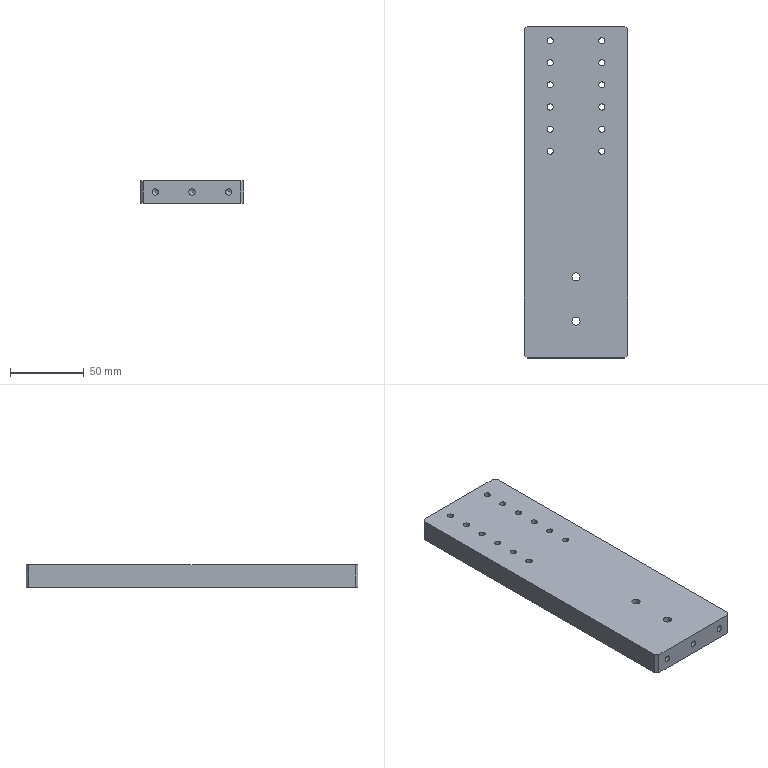Part | NX | 1 solid | 40 faces | box 70 x 225 x 15 mm | volume 210528 mm3 | cylinder 21 | plane 16 | cone 3 | commonest cylinder face diameters 4.2 x15 4 x2 5.5 x2 10 x2
STEP:
#1=CARTESIAN_POINT('',(-33.,112.5,15.));
#2=VERTEX_POINT('',#1);
#3=CARTESIAN_POINT('',(-35.,110.5,15.));
#4=VERTEX_POINT('',#3);
#5=CARTESIAN_POINT('',(-35.,110.5,15.));
#6=DIRECTION('',(-0.7071,-0.7071,0.));
#7=VECTOR('',#6,1000.);
#8=LINE('',#5,#7);
#9=EDGE_CURVE('',#2,#4,#8,.T.);
#10=ORIENTED_EDGE('',*,*,#9,.F.);
#11=CARTESIAN_POINT('',(-33.,112.5,0.));
#12=VERTEX_POINT('',#11);
#13=CARTESIAN_POINT('',(-33.,112.5,15.));
#14=DIRECTION('',(0.,0.,1.));
#15=VECTOR('',#14,1000.);
#16=LINE('',#13,#15);
#17=EDGE_CURVE('',#12,#2,#16,.T.);
#18=ORIENTED_EDGE('',*,*,#17,.F.);
#19=CARTESIAN_POINT('',(-35.,110.5,0.));
#20=VERTEX_POINT('',#19);
#21=CARTESIAN_POINT('',(-72.75,72.75,0.));
#22=DIRECTION('',(0.7071,0.7071,0.));
#23=VECTOR('',#22,1000.);
#24=LINE('',#21,#23);
#25=EDGE_CURVE('',#20,#12,#24,.T.);
#26=ORIENTED_EDGE('',*,*,#25,.F.);
#27=CARTESIAN_POINT('',(-35.,110.5,15.));
#28=DIRECTION('',(0.,0.,-1.));
#29=VECTOR('',#28,1000.);
#30=LINE('',#27,#29);
#31=EDGE_CURVE('',#4,#20,#30,.T.);
#32=ORIENTED_EDGE('',*,*,#31,.F.);
#33=EDGE_LOOP('',(#10,#18,#26,#32));
#34=FACE_BOUND('',#33,.T.);
#35=CARTESIAN_POINT('',(-35.,110.5,15.));
#36=DIRECTION('',(0.7071,-0.7071,0.));
#37=DIRECTION('',(0.,0.,-1.));
#38=AXIS2_PLACEMENT_3D('',#35,#36,#37);
#39=PLANE('',#38);
#40=ADVANCED_FACE('',(#34),#39,.F.);
#41=CARTESIAN_POINT('',(35.,110.5,15.));
#42=VERTEX_POINT('',#41);
#43=CARTESIAN_POINT('',(33.,112.5,15.));
#44=VERTEX_POINT('',#43);
#45=CARTESIAN_POINT('',(33.,112.5,15.));
#46=DIRECTION('',(-0.7071,0.7071,0.));
#47=VECTOR('',#46,1000.);
#48=LINE('',#45,#47);
#49=EDGE_CURVE('',#42,#44,#48,.T.);
#50=ORIENTED_EDGE('',*,*,#49,.F.);
#51=CARTESIAN_POINT('',(35.,110.5,0.));
#52=VERTEX_POINT('',#51);
#53=CARTESIAN_POINT('',(35.,110.5,15.));
#54=DIRECTION('',(0.,0.,1.));
#55=VECTOR('',#54,1000.);
#56=LINE('',#53,#55);
#57=EDGE_CURVE('',#52,#42,#56,.T.);
#58=ORIENTED_EDGE('',*,*,#57,.F.);
#59=CARTESIAN_POINT('',(33.,112.5,0.));
#60=VERTEX_POINT('',#59);
#61=CARTESIAN_POINT('',(72.75,72.75,0.));
#62=DIRECTION('',(0.7071,-0.7071,0.));
#63=VECTOR('',#62,1000.);
#64=LINE('',#61,#63);
#65=EDGE_CURVE('',#60,#52,#64,.T.);
#66=ORIENTED_EDGE('',*,*,#65,.F.);
#67=CARTESIAN_POINT('',(33.,112.5,15.));
#68=DIRECTION('',(0.,0.,-1.));
#69=VECTOR('',#68,1000.);
#70=LINE('',#67,#69);
#71=EDGE_CURVE('',#44,#60,#70,.T.);
#72=ORIENTED_EDGE('',*,*,#71,.F.);
#73=EDGE_LOOP('',(#50,#58,#66,#72));
#74=FACE_BOUND('',#73,.T.);
#75=CARTESIAN_POINT('',(33.,112.5,15.));
#76=DIRECTION('',(-0.7071,-0.7071,0.));
#77=DIRECTION('',(0.,0.,-1.));
#78=AXIS2_PLACEMENT_3D('',#75,#76,#77);
#79=PLANE('',#78);
#80=ADVANCED_FACE('',(#74),#79,.F.);
#81=CARTESIAN_POINT('',(-35.,-110.5,15.));
#82=VERTEX_POINT('',#81);
#83=CARTESIAN_POINT('',(-33.,-112.5,15.));
#84=VERTEX_POINT('',#83);
#85=CARTESIAN_POINT('',(-33.,-112.5,15.));
#86=DIRECTION('',(0.7071,-0.7071,0.));
#87=VECTOR('',#86,1000.);
#88=LINE('',#85,#87);
#89=EDGE_CURVE('',#82,#84,#88,.T.);
#90=ORIENTED_EDGE('',*,*,#89,.F.);
#91=CARTESIAN_POINT('',(-35.,-110.5,0.));
#92=VERTEX_POINT('',#91);
#93=CARTESIAN_POINT('',(-35.,-110.5,15.));
#94=DIRECTION('',(0.,0.,1.));
#95=VECTOR('',#94,1000.);
#96=LINE('',#93,#95);
#97=EDGE_CURVE('',#92,#82,#96,.T.);
#98=ORIENTED_EDGE('',*,*,#97,.F.);
#99=CARTESIAN_POINT('',(-33.,-112.5,0.));
#100=VERTEX_POINT('',#99);
#101=CARTESIAN_POINT('',(-72.75,-72.75,0.));
#102=DIRECTION('',(-0.7071,0.7071,0.));
#103=VECTOR('',#102,1000.);
#104=LINE('',#101,#103);
#105=EDGE_CURVE('',#100,#92,#104,.T.);
#106=ORIENTED_EDGE('',*,*,#105,.F.);
#107=CARTESIAN_POINT('',(-33.,-112.5,15.));
#108=DIRECTION('',(0.,0.,-1.));
#109=VECTOR('',#108,1000.);
#110=LINE('',#107,#109);
#111=EDGE_CURVE('',#84,#100,#110,.T.);
#112=ORIENTED_EDGE('',*,*,#111,.F.);
#113=EDGE_LOOP('',(#90,#98,#106,#112));
#114=FACE_BOUND('',#113,.T.);
#115=CARTESIAN_POINT('',(-33.,-112.5,15.));
#116=DIRECTION('',(0.7071,0.7071,0.));
#117=DIRECTION('',(0.,0.,-1.));
#118=AXIS2_PLACEMENT_3D('',#115,#116,#117);
#119=PLANE('',#118);
#120=ADVANCED_FACE('',(#114),#119,.F.);
#121=CARTESIAN_POINT('',(33.,-112.5,15.));
#122=VERTEX_POINT('',#121);
#123=CARTESIAN_POINT('',(35.,-110.5,15.));
#124=VERTEX_POINT('',#123);
#125=CARTESIAN_POINT('',(35.,-110.5,15.));
#126=DIRECTION('',(0.7071,0.7071,0.));
#127=VECTOR('',#126,1000.);
#128=LINE('',#125,#127);
#129=EDGE_CURVE('',#122,#124,#128,.T.);
#130=ORIENTED_EDGE('',*,*,#129,.F.);
#131=CARTESIAN_POINT('',(33.,-112.5,0.));
#132=VERTEX_POINT('',#131);
#133=CARTESIAN_POINT('',(33.,-112.5,15.));
#134=DIRECTION('',(0.,0.,1.));
#135=VECTOR('',#134,1000.);
#136=LINE('',#133,#135);
#137=EDGE_CURVE('',#132,#122,#136,.T.);
#138=ORIENTED_EDGE('',*,*,#137,.F.);
#139=CARTESIAN_POINT('',(35.,-110.5,0.));
#140=VERTEX_POINT('',#139);
#141=CARTESIAN_POINT('',(72.75,-72.75,0.));
#142=DIRECTION('',(-0.7071,-0.7071,0.));
#143=VECTOR('',#142,1000.);
#144=LINE('',#141,#143);
#145=EDGE_CURVE('',#140,#132,#144,.T.);
#146=ORIENTED_EDGE('',*,*,#145,.F.);
#147=CARTESIAN_POINT('',(35.,-110.5,15.));
#148=DIRECTION('',(0.,0.,-1.));
#149=VECTOR('',#148,1000.);
#150=LINE('',#147,#149);
#151=EDGE_CURVE('',#124,#140,#150,.T.);
#152=ORIENTED_EDGE('',*,*,#151,.F.);
#153=EDGE_LOOP('',(#130,#138,#146,#152));
#154=FACE_BOUND('',#153,.T.);
#155=CARTESIAN_POINT('',(35.,-110.5,15.));
#156=DIRECTION('',(-0.7071,0.7071,0.));
#157=DIRECTION('',(0.,0.,-1.));
#158=AXIS2_PLACEMENT_3D('',#155,#156,#157);
#159=PLANE('',#158);
#160=ADVANCED_FACE('',(#154),#159,.F.);
#161=CARTESIAN_POINT('',(-5.,-57.5,7.));
#162=VERTEX_POINT('',#161);
#163=CARTESIAN_POINT('',(0.,-57.5,7.));
#164=DIRECTION('',(0.,0.,-1.));
#165=DIRECTION('',(-1.,0.,0.));
#166=AXIS2_PLACEMENT_3D('',#163,#164,#165);
#167=CIRCLE('',#166,5.);
#168=EDGE_CURVE('',#162,#162,#167,.T.);
#169=ORIENTED_EDGE('',*,*,#168,.T.);
#170=EDGE_LOOP('',(#169));
#171=FACE_BOUND('',#170,.T.);
#172=CARTESIAN_POINT('',(-2.75,-57.5,7.));
#173=VERTEX_POINT('',#172);
#174=CARTESIAN_POINT('',(0.,-57.5,7.));
#175=DIRECTION('',(0.,0.,-1.));
#176=DIRECTION('',(-1.,0.,0.));
#177=AXIS2_PLACEMENT_3D('',#174,#175,#176);
#178=CIRCLE('',#177,2.75);
#179=EDGE_CURVE('',#173,#173,#178,.T.);
#180=ORIENTED_EDGE('',*,*,#179,.F.);
#181=EDGE_LOOP('',(#180));
#182=FACE_BOUND('',#181,.T.);
#183=CARTESIAN_POINT('',(2.75,-57.5,7.));
#184=DIRECTION('',(0.,0.,1.));
#185=DIRECTION('',(1.,0.,0.));
#186=AXIS2_PLACEMENT_3D('',#183,#184,#185);
#187=PLANE('',#186);
#188=ADVANCED_FACE('',(#171,#182),#187,.F.);
#189=CARTESIAN_POINT('',(5.,-87.5,7.));
#190=VERTEX_POINT('',#189);
#191=CARTESIAN_POINT('',(0.,-87.5,7.));
#192=DIRECTION('',(0.,0.,-1.));
#193=DIRECTION('',(1.,0.,0.));
#194=AXIS2_PLACEMENT_3D('',#191,#192,#193);
#195=CIRCLE('',#194,5.);
#196=EDGE_CURVE('',#190,#190,#195,.T.);
#197=ORIENTED_EDGE('',*,*,#196,.T.);
#198=EDGE_LOOP('',(#197));
#199=FACE_BOUND('',#198,.T.);
#200=CARTESIAN_POINT('',(2.75,-87.5,7.));
#201=VERTEX_POINT('',#200);
#202=CARTESIAN_POINT('',(0.,-87.5,7.));
#203=DIRECTION('',(0.,0.,-1.));
#204=DIRECTION('',(1.,0.,0.));
#205=AXIS2_PLACEMENT_3D('',#202,#203,#204);
#206=CIRCLE('',#205,2.75);
#207=EDGE_CURVE('',#201,#201,#206,.T.);
#208=ORIENTED_EDGE('',*,*,#207,.F.);
#209=EDGE_LOOP('',(#208));
#210=FACE_BOUND('',#209,.T.);
#211=CARTESIAN_POINT('',(2.75,-57.5,7.));
#212=DIRECTION('',(0.,0.,1.));
#213=DIRECTION('',(1.,0.,0.));
#214=AXIS2_PLACEMENT_3D('',#211,#212,#213);
#215=PLANE('',#214);
#216=ADVANCED_FACE('',(#199,#210),#215,.F.);
#217=CARTESIAN_POINT('',(30.,-5.5,3.));
#218=VERTEX_POINT('',#217);
#219=CARTESIAN_POINT('',(28.,-7.5,3.));
#220=VERTEX_POINT('',#219);
#221=CARTESIAN_POINT('',(28.,-5.5,3.));
#222=DIRECTION('',(0.,0.,-1.));
#223=DIRECTION('',(-1.,0.,0.));
#224=AXIS2_PLACEMENT_3D('',#221,#222,#223);
#225=CIRCLE('',#224,2.);
#226=EDGE_CURVE('',#218,#220,#225,.T.);
#227=ORIENTED_EDGE('',*,*,#226,.F.);
#228=CARTESIAN_POINT('',(30.,-5.5,0.));
#229=VERTEX_POINT('',#228);
#230=CARTESIAN_POINT('',(30.,-5.5,3.));
#231=DIRECTION('',(0.,0.,1.));
#232=VECTOR('',#231,1000.);
#233=LINE('',#230,#232);
#234=EDGE_CURVE('',#229,#218,#233,.T.);
#235=ORIENTED_EDGE('',*,*,#234,.F.);
#236=CARTESIAN_POINT('',(28.,-7.5,0.));
#237=VERTEX_POINT('',#236);
#238=CARTESIAN_POINT('',(28.,-5.5,0.));
#239=DIRECTION('',(0.,0.,1.));
#240=DIRECTION('',(-1.,0.,0.));
#241=AXIS2_PLACEMENT_3D('',#238,#239,#240);
#242=CIRCLE('',#241,2.);
#243=EDGE_CURVE('',#237,#229,#242,.T.);
#244=ORIENTED_EDGE('',*,*,#243,.F.);
#245=CARTESIAN_POINT('',(28.,-7.5,0.));
#246=DIRECTION('',(0.,0.,-1.));
#247=VECTOR('',#246,1000.);
#248=LINE('',#245,#247);
#249=EDGE_CURVE('',#220,#237,#248,.T.);
#250=ORIENTED_EDGE('',*,*,#249,.F.);
#251=EDGE_LOOP('',(#227,#235,#244,#250));
#252=FACE_BOUND('',#251,.T.);
#253=CARTESIAN_POINT('',(28.,-5.5,3.));
#254=DIRECTION('',(0.,0.,1.));
#255=DIRECTION('',(1.,0.,0.));
#256=AXIS2_PLACEMENT_3D('',#253,#254,#255);
#257=CYLINDRICAL_SURFACE('',#256,2.);
#258=ADVANCED_FACE('',(#252),#257,.F.);
#259=CARTESIAN_POINT('',(-28.,-7.5,3.));
#260=VERTEX_POINT('',#259);
#261=CARTESIAN_POINT('',(-30.,-5.5,3.));
#262=VERTEX_POINT('',#261);
#263=CARTESIAN_POINT('',(-28.,-5.5,3.));
#264=DIRECTION('',(0.,0.,-1.));
#265=DIRECTION('',(-1.,0.,0.));
#266=AXIS2_PLACEMENT_3D('',#263,#264,#265);
#267=CIRCLE('',#266,2.);
#268=EDGE_CURVE('',#260,#262,#267,.T.);
#269=ORIENTED_EDGE('',*,*,#268,.F.);
#270=CARTESIAN_POINT('',(-28.,-7.5,0.));
#271=VERTEX_POINT('',#270);
#272=CARTESIAN_POINT('',(-28.,-7.5,3.));
#273=DIRECTION('',(0.,0.,1.));
#274=VECTOR('',#273,1000.);
#275=LINE('',#272,#274);
#276=EDGE_CURVE('',#271,#260,#275,.T.);
#277=ORIENTED_EDGE('',*,*,#276,.F.);
#278=CARTESIAN_POINT('',(-30.,-5.5,0.));
#279=VERTEX_POINT('',#278);
#280=CARTESIAN_POINT('',(-28.,-5.5,0.));
#281=DIRECTION('',(0.,0.,1.));
#282=DIRECTION('',(-1.,0.,0.));
#283=AXIS2_PLACEMENT_3D('',#280,#281,#282);
#284=CIRCLE('',#283,2.);
#285=EDGE_CURVE('',#279,#271,#284,.T.);
#286=ORIENTED_EDGE('',*,*,#285,.F.);
#287=CARTESIAN_POINT('',(-30.,-5.5,0.));
#288=DIRECTION('',(0.,0.,-1.));
#289=VECTOR('',#288,1000.);
#290=LINE('',#287,#289);
#291=EDGE_CURVE('',#262,#279,#290,.T.);
#292=ORIENTED_EDGE('',*,*,#291,.F.);
#293=EDGE_LOOP('',(#269,#277,#286,#292));
#294=FACE_BOUND('',#293,.T.);
#295=CARTESIAN_POINT('',(-28.,-5.5,3.));
#296=DIRECTION('',(0.,0.,1.));
#297=DIRECTION('',(1.,0.,0.));
#298=AXIS2_PLACEMENT_3D('',#295,#296,#297);
#299=CYLINDRICAL_SURFACE('',#298,2.);
#300=ADVANCED_FACE('',(#294),#299,.F.);
#301=CARTESIAN_POINT('',(30.,-7.5,0.));
#302=DIRECTION('',(-1.,0.,0.));
#303=VECTOR('',#302,1000.);
#304=LINE('',#301,#303);
#305=EDGE_CURVE('',#237,#271,#304,.T.);
#306=ORIENTED_EDGE('',*,*,#305,.T.);
#307=ORIENTED_EDGE('',*,*,#276,.T.);
#308=CARTESIAN_POINT('',(30.,-7.5,3.));
#309=DIRECTION('',(-1.,0.,0.));
#310=VECTOR('',#309,1000.);
#311=LINE('',#308,#310);
#312=EDGE_CURVE('',#220,#260,#311,.T.);
#313=ORIENTED_EDGE('',*,*,#312,.F.);
#314=ORIENTED_EDGE('',*,*,#249,.T.);
#315=EDGE_LOOP('',(#306,#307,#313,#314));
#316=FACE_BOUND('',#315,.T.);
#317=CARTESIAN_POINT('',(30.,-7.5,3.));
#318=DIRECTION('',(0.,-1.,0.));
#319=DIRECTION('',(1.,0.,0.));
#320=AXIS2_PLACEMENT_3D('',#317,#318,#319);
#321=PLANE('',#320);
#322=ADVANCED_FACE('',(#316),#321,.F.);
#323=CARTESIAN_POINT('',(30.,112.5,0.));
#324=VERTEX_POINT('',#323);
#325=CARTESIAN_POINT('',(30.,0.,0.));
#326=DIRECTION('',(0.,-1.,0.));
#327=VECTOR('',#326,1000.);
#328=LINE('',#325,#327);
#329=EDGE_CURVE('',#324,#229,#328,.T.);
#330=ORIENTED_EDGE('',*,*,#329,.T.);
#331=ORIENTED_EDGE('',*,*,#234,.T.);
#332=CARTESIAN_POINT('',(30.,112.5,3.));
#333=VERTEX_POINT('',#332);
#334=CARTESIAN_POINT('',(30.,232.5,3.));
#335=DIRECTION('',(0.,-1.,0.));
#336=VECTOR('',#335,1000.);
#337=LINE('',#334,#336);
#338=EDGE_CURVE('',#333,#218,#337,.T.);
#339=ORIENTED_EDGE('',*,*,#338,.F.);
#340=CARTESIAN_POINT('',(30.,112.5,15.));
#341=DIRECTION('',(0.,0.,1.));
#342=VECTOR('',#341,1000.);
#343=LINE('',#340,#342);
#344=EDGE_CURVE('',#324,#333,#343,.T.);
#345=ORIENTED_EDGE('',*,*,#344,.F.);
#346=EDGE_LOOP('',(#330,#331,#339,#345));
#347=FACE_BOUND('',#346,.T.);
#348=CARTESIAN_POINT('',(30.,232.5,3.));
#349=DIRECTION('',(1.,0.,0.));
#350=DIRECTION('',(0.,0.,-1.));
#351=AXIS2_PLACEMENT_3D('',#348,#349,#350);
#352=PLANE('',#351);
#353=ADVANCED_FACE('',(#347),#352,.F.);
#354=CARTESIAN_POINT('',(-30.,112.5,3.));
#355=VERTEX_POINT('',#354);
#356=CARTESIAN_POINT('',(-30.,232.5,3.));
#357=DIRECTION('',(0.,1.,0.));
#358=VECTOR('',#357,1000.);
#359=LINE('',#356,#358);
#360=EDGE_CURVE('',#262,#355,#359,.T.);
#361=ORIENTED_EDGE('',*,*,#360,.F.);
#362=ORIENTED_EDGE('',*,*,#291,.T.);
#363=CARTESIAN_POINT('',(-30.,112.5,0.));
#364=VERTEX_POINT('',#363);
#365=CARTESIAN_POINT('',(-30.,232.5,0.));
#366=DIRECTION('',(0.,1.,0.));
#367=VECTOR('',#366,1000.);
#368=LINE('',#365,#367);
#369=EDGE_CURVE('',#279,#364,#368,.T.);
#370=ORIENTED_EDGE('',*,*,#369,.T.);
#371=CARTESIAN_POINT('',(-30.,112.5,15.));
#372=DIRECTION('',(0.,0.,-1.));
#373=VECTOR('',#372,1000.);
#374=LINE('',#371,#373);
#375=EDGE_CURVE('',#355,#364,#374,.T.);
#376=ORIENTED_EDGE('',*,*,#375,.F.);
#377=EDGE_LOOP('',(#361,#362,#370,#376));
#378=FACE_BOUND('',#377,.T.);
#379=CARTESIAN_POINT('',(-30.,232.5,3.));
#380=DIRECTION('',(-1.,0.,0.));
#381=DIRECTION('',(0.,-1.,0.));
#382=AXIS2_PLACEMENT_3D('',#379,#380,#381);
#383=PLANE('',#382);
#384=ADVANCED_FACE('',(#378),#383,.F.);
#385=ORIENTED_EDGE('',*,*,#312,.T.);
#386=ORIENTED_EDGE('',*,*,#268,.T.);
#387=ORIENTED_EDGE('',*,*,#360,.T.);
#388=CARTESIAN_POINT('',(-35.,112.5,3.));
#389=DIRECTION('',(1.,0.,0.));
#390=VECTOR('',#389,1000.);
#391=LINE('',#388,#390);
#392=EDGE_CURVE('',#355,#333,#391,.T.);
#393=ORIENTED_EDGE('',*,*,#392,.T.);
#394=ORIENTED_EDGE('',*,*,#338,.T.);
#395=ORIENTED_EDGE('',*,*,#226,.T.);
#396=EDGE_LOOP('',(#385,#386,#387,#393,#394,#395));
#397=FACE_BOUND('',#396,.T.);
#398=CARTESIAN_POINT('',(-19.6,102.571,3.));
#399=VERTEX_POINT('',#398);
#400=CARTESIAN_POINT('',(-17.5,102.571,3.));
#401=DIRECTION('',(0.,0.,-1.));
#402=DIRECTION('',(-1.,0.,0.));
#403=AXIS2_PLACEMENT_3D('',#400,#401,#402);
#404=CIRCLE('',#403,2.1);
#405=EDGE_CURVE('',#399,#399,#404,.T.);
#406=ORIENTED_EDGE('',*,*,#405,.F.);
#407=EDGE_LOOP('',(#406));
#408=FACE_BOUND('',#407,.T.);
#409=CARTESIAN_POINT('',(15.4,102.571,3.));
#410=VERTEX_POINT('',#409);
#411=CARTESIAN_POINT('',(17.5,102.571,3.));
#412=DIRECTION('',(0.,0.,-1.));
#413=DIRECTION('',(-1.,0.,0.));
#414=AXIS2_PLACEMENT_3D('',#411,#412,#413);
#415=CIRCLE('',#414,2.1);
#416=EDGE_CURVE('',#410,#410,#415,.T.);
#417=ORIENTED_EDGE('',*,*,#416,.F.);
#418=EDGE_LOOP('',(#417));
#419=FACE_BOUND('',#418,.T.);
#420=CARTESIAN_POINT('',(-19.6,87.571,3.));
#421=VERTEX_POINT('',#420);
#422=CARTESIAN_POINT('',(-17.5,87.571,3.));
#423=DIRECTION('',(0.,0.,-1.));
#424=DIRECTION('',(-1.,0.,0.));
#425=AXIS2_PLACEMENT_3D('',#422,#423,#424);
#426=CIRCLE('',#425,2.1);
#427=EDGE_CURVE('',#421,#421,#426,.T.);
#428=ORIENTED_EDGE('',*,*,#427,.F.);
#429=EDGE_LOOP('',(#428));
#430=FACE_BOUND('',#429,.T.);
#431=CARTESIAN_POINT('',(15.4,87.571,3.));
#432=VERTEX_POINT('',#431);
#433=CARTESIAN_POINT('',(17.5,87.571,3.));
#434=DIRECTION('',(0.,0.,-1.));
#435=DIRECTION('',(-1.,0.,0.));
#436=AXIS2_PLACEMENT_3D('',#433,#434,#435);
#437=CIRCLE('',#436,2.1);
#438=EDGE_CURVE('',#432,#432,#437,.T.);
#439=ORIENTED_EDGE('',*,*,#438,.F.);
#440=EDGE_LOOP('',(#439));
#441=FACE_BOUND('',#440,.T.);
#442=CARTESIAN_POINT('',(-19.6,72.571,3.));
#443=VERTEX_POINT('',#442);
#444=CARTESIAN_POINT('',(-17.5,72.571,3.));
#445=DIRECTION('',(0.,0.,-1.));
#446=DIRECTION('',(-1.,0.,0.));
#447=AXIS2_PLACEMENT_3D('',#444,#445,#446);
#448=CIRCLE('',#447,2.1);
#449=EDGE_CURVE('',#443,#443,#448,.T.);
#450=ORIENTED_EDGE('',*,*,#449,.F.);
#451=EDGE_LOOP('',(#450));
#452=FACE_BOUND('',#451,.T.);
#453=CARTESIAN_POINT('',(15.4,72.571,3.));
#454=VERTEX_POINT('',#453);
#455=CARTESIAN_POINT('',(17.5,72.571,3.));
#456=DIRECTION('',(0.,0.,-1.));
#457=DIRECTION('',(-1.,0.,0.));
#458=AXIS2_PLACEMENT_3D('',#455,#456,#457);
#459=CIRCLE('',#458,2.1);
#460=EDGE_CURVE('',#454,#454,#459,.T.);
#461=ORIENTED_EDGE('',*,*,#460,.F.);
#462=EDGE_LOOP('',(#461));
#463=FACE_BOUND('',#462,.T.);
#464=CARTESIAN_POINT('',(-19.6,57.571,3.));
#465=VERTEX_POINT('',#464);
#466=CARTESIAN_POINT('',(-17.5,57.571,3.));
#467=DIRECTION('',(0.,0.,-1.));
#468=DIRECTION('',(-1.,0.,0.));
#469=AXIS2_PLACEMENT_3D('',#466,#467,#468);
#470=CIRCLE('',#469,2.1);
#471=EDGE_CURVE('',#465,#465,#470,.T.);
#472=ORIENTED_EDGE('',*,*,#471,.F.);
#473=EDGE_LOOP('',(#472));
#474=FACE_BOUND('',#473,.T.);
#475=CARTESIAN_POINT('',(15.4,57.571,3.));
#476=VERTEX_POINT('',#475);
#477=CARTESIAN_POINT('',(17.5,57.571,3.));
#478=DIRECTION('',(0.,0.,-1.));
#479=DIRECTION('',(-1.,0.,0.));
#480=AXIS2_PLACEMENT_3D('',#477,#478,#479);
#481=CIRCLE('',#480,2.1);
#482=EDGE_CURVE('',#476,#476,#481,.T.);
#483=ORIENTED_EDGE('',*,*,#482,.F.);
#484=EDGE_LOOP('',(#483));
#485=FACE_BOUND('',#484,.T.);
#486=CARTESIAN_POINT('',(-19.6,42.571,3.));
#487=VERTEX_POINT('',#486);
#488=CARTESIAN_POINT('',(-17.5,42.571,3.));
#489=DIRECTION('',(0.,0.,-1.));
#490=DIRECTION('',(-1.,0.,0.));
#491=AXIS2_PLACEMENT_3D('',#488,#489,#490);
#492=CIRCLE('',#491,2.1);
#493=EDGE_CURVE('',#487,#487,#492,.T.);
#494=ORIENTED_EDGE('',*,*,#493,.F.);
#495=EDGE_LOOP('',(#494));
#496=FACE_BOUND('',#495,.T.);
#497=CARTESIAN_POINT('',(15.4,42.571,3.));
#498=VERTEX_POINT('',#497);
#499=CARTESIAN_POINT('',(17.5,42.571,3.));
#500=DIRECTION('',(0.,0.,-1.));
#501=DIRECTION('',(-1.,0.,0.));
#502=AXIS2_PLACEMENT_3D('',#499,#500,#501);
#503=CIRCLE('',#502,2.1);
#504=EDGE_CURVE('',#498,#498,#503,.T.);
#505=ORIENTED_EDGE('',*,*,#504,.F.);
#506=EDGE_LOOP('',(#505));
#507=FACE_BOUND('',#506,.T.);
#508=CARTESIAN_POINT('',(-19.6,27.571,3.));
#509=VERTEX_POINT('',#508);
#510=CARTESIAN_POINT('',(-17.5,27.571,3.));
#511=DIRECTION('',(0.,0.,-1.));
#512=DIRECTION('',(-1.,0.,0.));
#513=AXIS2_PLACEMENT_3D('',#510,#511,#512);
#514=CIRCLE('',#513,2.1);
#515=EDGE_CURVE('',#509,#509,#514,.T.);
#516=ORIENTED_EDGE('',*,*,#515,.F.);
#517=EDGE_LOOP('',(#516));
#518=FACE_BOUND('',#517,.T.);
#519=CARTESIAN_POINT('',(15.4,27.571,3.));
#520=VERTEX_POINT('',#519);
#521=CARTESIAN_POINT('',(17.5,27.571,3.));
#522=DIRECTION('',(0.,0.,-1.));
#523=DIRECTION('',(-1.,0.,0.));
#524=AXIS2_PLACEMENT_3D('',#521,#522,#523);
#525=CIRCLE('',#524,2.1);
#526=EDGE_CURVE('',#520,#520,#525,.T.);
#527=ORIENTED_EDGE('',*,*,#526,.F.);
#528=EDGE_LOOP('',(#527));
#529=FACE_BOUND('',#528,.T.);
#530=CARTESIAN_POINT('',(0.,0.,3.));
#531=DIRECTION('',(0.,0.,-1.));
#532=DIRECTION('',(-1.,0.,0.));
#533=AXIS2_PLACEMENT_3D('',#530,#531,#532);
#534=PLANE('',#533);
#535=ADVANCED_FACE('',(#397,#408,#419,#430,#441,#452,#463,#474,#485,#496,#507,#518,#529),#534,.T.);
#536=CARTESIAN_POINT('',(35.,-112.5,0.));
#537=DIRECTION('',(0.,1.,0.));
#538=VECTOR('',#537,1000.);
#539=LINE('',#536,#538);
#540=EDGE_CURVE('',#140,#52,#539,.T.);
#541=ORIENTED_EDGE('',*,*,#540,.F.);
#542=ORIENTED_EDGE('',*,*,#145,.T.);
#543=CARTESIAN_POINT('',(-35.,-112.5,0.));
#544=DIRECTION('',(1.,0.,0.));
#545=VECTOR('',#544,1000.);
#546=LINE('',#543,#545);
#547=EDGE_CURVE('',#100,#132,#546,.T.);
#548=ORIENTED_EDGE('',*,*,#547,.F.);
#549=ORIENTED_EDGE('',*,*,#105,.T.);
#550=CARTESIAN_POINT('',(-35.,-112.5,0.));
#551=DIRECTION('',(0.,-1.,0.));
#552=VECTOR('',#551,1000.);
#553=LINE('',#550,#552);
#554=EDGE_CURVE('',#20,#92,#553,.T.);
#555=ORIENTED_EDGE('',*,*,#554,.F.);
#556=ORIENTED_EDGE('',*,*,#25,.T.);
#557=CARTESIAN_POINT('',(-35.,112.5,0.));
#558=DIRECTION('',(-1.,0.,0.));
#559=VECTOR('',#558,1000.);
#560=LINE('',#557,#559);
#561=EDGE_CURVE('',#364,#12,#560,.T.);
#562=ORIENTED_EDGE('',*,*,#561,.F.);
#563=ORIENTED_EDGE('',*,*,#369,.F.);
#564=ORIENTED_EDGE('',*,*,#285,.T.);
#565=ORIENTED_EDGE('',*,*,#305,.F.);
#566=ORIENTED_EDGE('',*,*,#243,.T.);
#567=ORIENTED_EDGE('',*,*,#329,.F.);
#568=CARTESIAN_POINT('',(-35.,112.5,0.));
#569=DIRECTION('',(-1.,0.,0.));
#570=VECTOR('',#569,1000.);
#571=LINE('',#568,#570);
#572=EDGE_CURVE('',#60,#324,#571,.T.);
#573=ORIENTED_EDGE('',*,*,#572,.F.);
#574=ORIENTED_EDGE('',*,*,#65,.T.);
#575=EDGE_LOOP('',(#541,#542,#548,#549,#555,#556,#562,#563,#564,#565,#566,#567,#573,#574));
#576=FACE_BOUND('',#575,.T.);
#577=CARTESIAN_POINT('',(-5.,-87.5,0.));
#578=VERTEX_POINT('',#577);
#579=CARTESIAN_POINT('',(0.,-87.5,0.));
#580=DIRECTION('',(0.,0.,-1.));
#581=DIRECTION('',(-1.,0.,0.));
#582=AXIS2_PLACEMENT_3D('',#579,#580,#581);
#583=CIRCLE('',#582,5.);
#584=EDGE_CURVE('',#578,#578,#583,.T.);
#585=ORIENTED_EDGE('',*,*,#584,.F.);
#586=EDGE_LOOP('',(#585));
#587=FACE_BOUND('',#586,.T.);
#588=CARTESIAN_POINT('',(-5.,-57.5,0.));
#589=VERTEX_POINT('',#588);
#590=CARTESIAN_POINT('',(0.,-57.5,0.));
#591=DIRECTION('',(0.,0.,-1.));
#592=DIRECTION('',(-1.,0.,0.));
#593=AXIS2_PLACEMENT_3D('',#590,#591,#592);
#594=CIRCLE('',#593,5.);
#595=EDGE_CURVE('',#589,#589,#594,.T.);
#596=ORIENTED_EDGE('',*,*,#595,.F.);
#597=EDGE_LOOP('',(#596));
#598=FACE_BOUND('',#597,.T.);
#599=CARTESIAN_POINT('',(0.,0.,0.));
#600=DIRECTION('',(0.,0.,-1.));
#601=DIRECTION('',(-1.,0.,0.));
#602=AXIS2_PLACEMENT_3D('',#599,#600,#601);
#603=PLANE('',#602);
#604=ADVANCED_FACE('',(#576,#587,#598),#603,.T.);
#605=CARTESIAN_POINT('',(-35.,-112.5,15.));
#606=DIRECTION('',(1.,0.,0.));
#607=VECTOR('',#606,1000.);
#608=LINE('',#605,#607);
#609=EDGE_CURVE('',#84,#122,#608,.T.);
#610=ORIENTED_EDGE('',*,*,#609,.T.);
#611=ORIENTED_EDGE('',*,*,#129,.T.);
#612=CARTESIAN_POINT('',(35.,-112.5,15.));
#613=DIRECTION('',(0.,1.,0.));
#614=VECTOR('',#613,1000.);
#615=LINE('',#612,#614);
#616=EDGE_CURVE('',#124,#42,#615,.T.);
#617=ORIENTED_EDGE('',*,*,#616,.T.);
#618=ORIENTED_EDGE('',*,*,#49,.T.);
#619=CARTESIAN_POINT('',(-35.,112.5,15.));
#620=DIRECTION('',(-1.,0.,0.));
#621=VECTOR('',#620,1000.);
#622=LINE('',#619,#621);
#623=EDGE_CURVE('',#44,#2,#622,.T.);
#624=ORIENTED_EDGE('',*,*,#623,.T.);
#625=ORIENTED_EDGE('',*,*,#9,.T.);
#626=CARTESIAN_POINT('',(-35.,-112.5,15.));
#627=DIRECTION('',(0.,-1.,0.));
#628=VECTOR('',#627,1000.);
#629=LINE('',#626,#628);
#630=EDGE_CURVE('',#4,#82,#629,.T.);
#631=ORIENTED_EDGE('',*,*,#630,.T.);
#632=ORIENTED_EDGE('',*,*,#89,.T.);
#633=EDGE_LOOP('',(#610,#611,#617,#618,#624,#625,#631,#632));
#634=FACE_BOUND('',#633,.T.);
#635=CARTESIAN_POINT('',(-19.6,102.571,15.));
#636=VERTEX_POINT('',#635);
#637=CARTESIAN_POINT('',(-17.5,102.571,15.));
#638=DIRECTION('',(0.,0.,-1.));
#639=DIRECTION('',(-1.,0.,0.));
#640=AXIS2_PLACEMENT_3D('',#637,#638,#639);
#641=CIRCLE('',#640,2.1);
#642=EDGE_CURVE('',#636,#636,#641,.T.);
#643=ORIENTED_EDGE('',*,*,#642,.T.);
#644=EDGE_LOOP('',(#643));
#645=FACE_BOUND('',#644,.T.);
#646=CARTESIAN_POINT('',(15.4,102.571,15.));
#647=VERTEX_POINT('',#646);
#648=CARTESIAN_POINT('',(17.5,102.571,15.));
#649=DIRECTION('',(0.,0.,-1.));
#650=DIRECTION('',(-1.,0.,0.));
#651=AXIS2_PLACEMENT_3D('',#648,#649,#650);
#652=CIRCLE('',#651,2.1);
#653=EDGE_CURVE('',#647,#647,#652,.T.);
#654=ORIENTED_EDGE('',*,*,#653,.T.);
#655=EDGE_LOOP('',(#654));
#656=FACE_BOUND('',#655,.T.);
#657=CARTESIAN_POINT('',(-19.6,87.571,15.));
#658=VERTEX_POINT('',#657);
#659=CARTESIAN_POINT('',(-17.5,87.571,15.));
#660=DIRECTION('',(0.,0.,-1.));
#661=DIRECTION('',(-1.,0.,0.));
#662=AXIS2_PLACEMENT_3D('',#659,#660,#661);
#663=CIRCLE('',#662,2.1);
#664=EDGE_CURVE('',#658,#658,#663,.T.);
#665=ORIENTED_EDGE('',*,*,#664,.T.);
#666=EDGE_LOOP('',(#665));
#667=FACE_BOUND('',#666,.T.);
#668=CARTESIAN_POINT('',(15.4,87.571,15.));
#669=VERTEX_POINT('',#668);
#670=CARTESIAN_POINT('',(17.5,87.571,15.));
#671=DIRECTION('',(0.,0.,-1.));
#672=DIRECTION('',(-1.,0.,0.));
#673=AXIS2_PLACEMENT_3D('',#670,#671,#672);
#674=CIRCLE('',#673,2.1);
#675=EDGE_CURVE('',#669,#669,#674,.T.);
#676=ORIENTED_EDGE('',*,*,#675,.T.);
#677=EDGE_LOOP('',(#676));
#678=FACE_BOUND('',#677,.T.);
#679=CARTESIAN_POINT('',(-19.6,72.571,15.));
#680=VERTEX_POINT('',#679);
#681=CARTESIAN_POINT('',(-17.5,72.571,15.));
#682=DIRECTION('',(0.,0.,-1.));
#683=DIRECTION('',(-1.,0.,0.));
#684=AXIS2_PLACEMENT_3D('',#681,#682,#683);
#685=CIRCLE('',#684,2.1);
#686=EDGE_CURVE('',#680,#680,#685,.T.);
#687=ORIENTED_EDGE('',*,*,#686,.T.);
#688=EDGE_LOOP('',(#687));
#689=FACE_BOUND('',#688,.T.);
#690=CARTESIAN_POINT('',(15.4,72.571,15.));
#691=VERTEX_POINT('',#690);
#692=CARTESIAN_POINT('',(17.5,72.571,15.));
#693=DIRECTION('',(0.,0.,-1.));
#694=DIRECTION('',(-1.,0.,0.));
#695=AXIS2_PLACEMENT_3D('',#692,#693,#694);
#696=CIRCLE('',#695,2.1);
#697=EDGE_CURVE('',#691,#691,#696,.T.);
#698=ORIENTED_EDGE('',*,*,#697,.T.);
#699=EDGE_LOOP('',(#698));
#700=FACE_BOUND('',#699,.T.);
#701=CARTESIAN_POINT('',(-19.6,57.571,15.));
#702=VERTEX_POINT('',#701);
#703=CARTESIAN_POINT('',(-17.5,57.571,15.));
#704=DIRECTION('',(0.,0.,-1.));
#705=DIRECTION('',(-1.,0.,0.));
#706=AXIS2_PLACEMENT_3D('',#703,#704,#705);
#707=CIRCLE('',#706,2.1);
#708=EDGE_CURVE('',#702,#702,#707,.T.);
#709=ORIENTED_EDGE('',*,*,#708,.T.);
#710=EDGE_LOOP('',(#709));
#711=FACE_BOUND('',#710,.T.);
#712=CARTESIAN_POINT('',(15.4,57.571,15.));
#713=VERTEX_POINT('',#712);
#714=CARTESIAN_POINT('',(17.5,57.571,15.));
#715=DIRECTION('',(0.,0.,-1.));
#716=DIRECTION('',(-1.,0.,0.));
#717=AXIS2_PLACEMENT_3D('',#714,#715,#716);
#718=CIRCLE('',#717,2.1);
#719=EDGE_CURVE('',#713,#713,#718,.T.);
#720=ORIENTED_EDGE('',*,*,#719,.T.);
#721=EDGE_LOOP('',(#720));
#722=FACE_BOUND('',#721,.T.);
#723=CARTESIAN_POINT('',(-19.6,42.571,15.));
#724=VERTEX_POINT('',#723);
#725=CARTESIAN_POINT('',(-17.5,42.571,15.));
#726=DIRECTION('',(0.,0.,-1.));
#727=DIRECTION('',(-1.,0.,0.));
#728=AXIS2_PLACEMENT_3D('',#725,#726,#727);
#729=CIRCLE('',#728,2.1);
#730=EDGE_CURVE('',#724,#724,#729,.T.);
#731=ORIENTED_EDGE('',*,*,#730,.T.);
#732=EDGE_LOOP('',(#731));
#733=FACE_BOUND('',#732,.T.);
#734=CARTESIAN_POINT('',(15.4,42.571,15.));
#735=VERTEX_POINT('',#734);
#736=CARTESIAN_POINT('',(17.5,42.571,15.));
#737=DIRECTION('',(0.,0.,-1.));
#738=DIRECTION('',(-1.,0.,0.));
#739=AXIS2_PLACEMENT_3D('',#736,#737,#738);
#740=CIRCLE('',#739,2.1);
#741=EDGE_CURVE('',#735,#735,#740,.T.);
#742=ORIENTED_EDGE('',*,*,#741,.T.);
#743=EDGE_LOOP('',(#742));
#744=FACE_BOUND('',#743,.T.);
#745=CARTESIAN_POINT('',(-19.6,27.571,15.));
#746=VERTEX_POINT('',#745);
#747=CARTESIAN_POINT('',(-17.5,27.571,15.));
#748=DIRECTION('',(0.,0.,-1.));
#749=DIRECTION('',(-1.,0.,0.));
#750=AXIS2_PLACEMENT_3D('',#747,#748,#749);
#751=CIRCLE('',#750,2.1);
#752=EDGE_CURVE('',#746,#746,#751,.T.);
#753=ORIENTED_EDGE('',*,*,#752,.T.);
#754=EDGE_LOOP('',(#753));
#755=FACE_BOUND('',#754,.T.);
#756=CARTESIAN_POINT('',(15.4,27.571,15.));
#757=VERTEX_POINT('',#756);
#758=CARTESIAN_POINT('',(17.5,27.571,15.));
#759=DIRECTION('',(0.,0.,-1.));
#760=DIRECTION('',(-1.,0.,0.));
#761=AXIS2_PLACEMENT_3D('',#758,#759,#760);
#762=CIRCLE('',#761,2.1);
#763=EDGE_CURVE('',#757,#757,#762,.T.);
#764=ORIENTED_EDGE('',*,*,#763,.T.);
#765=EDGE_LOOP('',(#764));
#766=FACE_BOUND('',#765,.T.);
#767=CARTESIAN_POINT('',(-2.75,-87.5,15.));
#768=VERTEX_POINT('',#767);
#769=CARTESIAN_POINT('',(0.,-87.5,15.));
#770=DIRECTION('',(0.,0.,-1.));
#771=DIRECTION('',(-1.,0.,0.));
#772=AXIS2_PLACEMENT_3D('',#769,#770,#771);
#773=CIRCLE('',#772,2.75);
#774=EDGE_CURVE('',#768,#768,#773,.T.);
#775=ORIENTED_EDGE('',*,*,#774,.T.);
#776=EDGE_LOOP('',(#775));
#777=FACE_BOUND('',#776,.T.);
#778=CARTESIAN_POINT('',(-2.75,-57.5,15.));
#779=VERTEX_POINT('',#778);
#780=CARTESIAN_POINT('',(0.,-57.5,15.));
#781=DIRECTION('',(0.,0.,-1.));
#782=DIRECTION('',(-1.,0.,0.));
#783=AXIS2_PLACEMENT_3D('',#780,#781,#782);
#784=CIRCLE('',#783,2.75);
#785=EDGE_CURVE('',#779,#779,#784,.T.);
#786=ORIENTED_EDGE('',*,*,#785,.T.);
#787=EDGE_LOOP('',(#786));
#788=FACE_BOUND('',#787,.T.);
#789=CARTESIAN_POINT('',(0.,0.,15.));
#790=DIRECTION('',(0.,0.,-1.));
#791=DIRECTION('',(-1.,0.,0.));
#792=AXIS2_PLACEMENT_3D('',#789,#790,#791);
#793=PLANE('',#792);
#794=ADVANCED_FACE('',(#634,#645,#656,#667,#678,#689,#700,#711,#722,#733,#744,#755,#766,#777,#788),#793,.F.);
#795=ORIENTED_EDGE('',*,*,#547,.T.);
#796=ORIENTED_EDGE('',*,*,#137,.T.);
#797=ORIENTED_EDGE('',*,*,#609,.F.);
#798=ORIENTED_EDGE('',*,*,#111,.T.);
#799=EDGE_LOOP('',(#795,#796,#797,#798));
#800=FACE_BOUND('',#799,.T.);
#801=CARTESIAN_POINT('',(0.,-112.5,5.4));
#802=VERTEX_POINT('',#801);
#803=CARTESIAN_POINT('',(0.,-112.5,7.5));
#804=DIRECTION('',(0.,-1.,0.));
#805=DIRECTION('',(0.,0.,-1.));
#806=AXIS2_PLACEMENT_3D('',#803,#804,#805);
#807=CIRCLE('',#806,2.1);
#808=EDGE_CURVE('',#802,#802,#807,.T.);
#809=ORIENTED_EDGE('',*,*,#808,.F.);
#810=EDGE_LOOP('',(#809));
#811=FACE_BOUND('',#810,.T.);
#812=CARTESIAN_POINT('',(25.,-112.5,5.4));
#813=VERTEX_POINT('',#812);
#814=CARTESIAN_POINT('',(25.,-112.5,7.5));
#815=DIRECTION('',(0.,-1.,0.));
#816=DIRECTION('',(0.,0.,-1.));
#817=AXIS2_PLACEMENT_3D('',#814,#815,#816);
#818=CIRCLE('',#817,2.1);
#819=EDGE_CURVE('',#813,#813,#818,.T.);
#820=ORIENTED_EDGE('',*,*,#819,.F.);
#821=EDGE_LOOP('',(#820));
#822=FACE_BOUND('',#821,.T.);
#823=CARTESIAN_POINT('',(-25.,-112.5,5.4));
#824=VERTEX_POINT('',#823);
#825=CARTESIAN_POINT('',(-25.,-112.5,7.5));
#826=DIRECTION('',(0.,-1.,0.));
#827=DIRECTION('',(0.,0.,-1.));
#828=AXIS2_PLACEMENT_3D('',#825,#826,#827);
#829=CIRCLE('',#828,2.1);
#830=EDGE_CURVE('',#824,#824,#829,.T.);
#831=ORIENTED_EDGE('',*,*,#830,.F.);
#832=EDGE_LOOP('',(#831));
#833=FACE_BOUND('',#832,.T.);
#834=CARTESIAN_POINT('',(-35.,-112.5,15.));
#835=DIRECTION('',(0.,1.,0.));
#836=DIRECTION('',(0.,0.,1.));
#837=AXIS2_PLACEMENT_3D('',#834,#835,#836);
#838=PLANE('',#837);
#839=ADVANCED_FACE('',(#800,#811,#822,#833),#838,.F.);
#840=ORIENTED_EDGE('',*,*,#554,.T.);
#841=ORIENTED_EDGE('',*,*,#97,.T.);
#842=ORIENTED_EDGE('',*,*,#630,.F.);
#843=ORIENTED_EDGE('',*,*,#31,.T.);
#844=EDGE_LOOP('',(#840,#841,#842,#843));
#845=FACE_BOUND('',#844,.T.);
#846=CARTESIAN_POINT('',(-35.,-112.5,15.));
#847=DIRECTION('',(1.,0.,0.));
#848=DIRECTION('',(0.,0.,-1.));
#849=AXIS2_PLACEMENT_3D('',#846,#847,#848);
#850=PLANE('',#849);
#851=ADVANCED_FACE('',(#845),#850,.F.);
#852=ORIENTED_EDGE('',*,*,#623,.F.);
#853=ORIENTED_EDGE('',*,*,#71,.T.);
#854=ORIENTED_EDGE('',*,*,#572,.T.);
#855=ORIENTED_EDGE('',*,*,#344,.T.);
#856=ORIENTED_EDGE('',*,*,#392,.F.);
#857=ORIENTED_EDGE('',*,*,#375,.T.);
#858=ORIENTED_EDGE('',*,*,#561,.T.);
#859=ORIENTED_EDGE('',*,*,#17,.T.);
#860=EDGE_LOOP('',(#852,#853,#854,#855,#856,#857,#858,#859));
#861=FACE_BOUND('',#860,.T.);
#862=CARTESIAN_POINT('',(-35.,112.5,15.));
#863=DIRECTION('',(0.,-1.,0.));
#864=DIRECTION('',(0.,0.,-1.));
#865=AXIS2_PLACEMENT_3D('',#862,#863,#864);
#866=PLANE('',#865);
#867=ADVANCED_FACE('',(#861),#866,.F.);
#868=ORIENTED_EDGE('',*,*,#616,.F.);
#869=ORIENTED_EDGE('',*,*,#151,.T.);
#870=ORIENTED_EDGE('',*,*,#540,.T.);
#871=ORIENTED_EDGE('',*,*,#57,.T.);
#872=EDGE_LOOP('',(#868,#869,#870,#871));
#873=FACE_BOUND('',#872,.T.);
#874=CARTESIAN_POINT('',(35.,-112.5,15.));
#875=DIRECTION('',(-1.,0.,0.));
#876=DIRECTION('',(0.,0.,1.));
#877=AXIS2_PLACEMENT_3D('',#874,#875,#876);
#878=PLANE('',#877);
#879=ADVANCED_FACE('',(#873),#878,.F.);
#880=ORIENTED_EDGE('',*,*,#405,.T.);
#881=EDGE_LOOP('',(#880));
#882=FACE_BOUND('',#881,.T.);
#883=ORIENTED_EDGE('',*,*,#642,.F.);
#884=EDGE_LOOP('',(#883));
#885=FACE_BOUND('',#884,.T.);
#886=CARTESIAN_POINT('',(-17.5,102.571,0.));
#887=DIRECTION('',(0.,0.,-1.));
#888=DIRECTION('',(-1.,0.,0.));
#889=AXIS2_PLACEMENT_3D('',#886,#887,#888);
#890=CYLINDRICAL_SURFACE('',#889,2.1);
#891=ADVANCED_FACE('',(#882,#885),#890,.F.);
#892=ORIENTED_EDGE('',*,*,#416,.T.);
#893=EDGE_LOOP('',(#892));
#894=FACE_BOUND('',#893,.T.);
#895=ORIENTED_EDGE('',*,*,#653,.F.);
#896=EDGE_LOOP('',(#895));
#897=FACE_BOUND('',#896,.T.);
#898=CARTESIAN_POINT('',(17.5,102.571,0.));
#899=DIRECTION('',(0.,0.,-1.));
#900=DIRECTION('',(-1.,0.,0.));
#901=AXIS2_PLACEMENT_3D('',#898,#899,#900);
#902=CYLINDRICAL_SURFACE('',#901,2.1);
#903=ADVANCED_FACE('',(#894,#897),#902,.F.);
#904=ORIENTED_EDGE('',*,*,#427,.T.);
#905=EDGE_LOOP('',(#904));
#906=FACE_BOUND('',#905,.T.);
#907=ORIENTED_EDGE('',*,*,#664,.F.);
#908=EDGE_LOOP('',(#907));
#909=FACE_BOUND('',#908,.T.);
#910=CARTESIAN_POINT('',(-17.5,87.571,0.));
#911=DIRECTION('',(0.,0.,-1.));
#912=DIRECTION('',(-1.,0.,0.));
#913=AXIS2_PLACEMENT_3D('',#910,#911,#912);
#914=CYLINDRICAL_SURFACE('',#913,2.1);
#915=ADVANCED_FACE('',(#906,#909),#914,.F.);
#916=ORIENTED_EDGE('',*,*,#438,.T.);
#917=EDGE_LOOP('',(#916));
#918=FACE_BOUND('',#917,.T.);
#919=ORIENTED_EDGE('',*,*,#675,.F.);
#920=EDGE_LOOP('',(#919));
#921=FACE_BOUND('',#920,.T.);
#922=CARTESIAN_POINT('',(17.5,87.571,0.));
#923=DIRECTION('',(0.,0.,-1.));
#924=DIRECTION('',(-1.,0.,0.));
#925=AXIS2_PLACEMENT_3D('',#922,#923,#924);
#926=CYLINDRICAL_SURFACE('',#925,2.1);
#927=ADVANCED_FACE('',(#918,#921),#926,.F.);
#928=ORIENTED_EDGE('',*,*,#449,.T.);
#929=EDGE_LOOP('',(#928));
#930=FACE_BOUND('',#929,.T.);
#931=ORIENTED_EDGE('',*,*,#686,.F.);
#932=EDGE_LOOP('',(#931));
#933=FACE_BOUND('',#932,.T.);
#934=CARTESIAN_POINT('',(-17.5,72.571,0.));
#935=DIRECTION('',(0.,0.,-1.));
#936=DIRECTION('',(-1.,0.,0.));
#937=AXIS2_PLACEMENT_3D('',#934,#935,#936);
#938=CYLINDRICAL_SURFACE('',#937,2.1);
#939=ADVANCED_FACE('',(#930,#933),#938,.F.);
#940=ORIENTED_EDGE('',*,*,#460,.T.);
#941=EDGE_LOOP('',(#940));
#942=FACE_BOUND('',#941,.T.);
#943=ORIENTED_EDGE('',*,*,#697,.F.);
#944=EDGE_LOOP('',(#943));
#945=FACE_BOUND('',#944,.T.);
#946=CARTESIAN_POINT('',(17.5,72.571,0.));
#947=DIRECTION('',(0.,0.,-1.));
#948=DIRECTION('',(-1.,0.,0.));
#949=AXIS2_PLACEMENT_3D('',#946,#947,#948);
#950=CYLINDRICAL_SURFACE('',#949,2.1);
#951=ADVANCED_FACE('',(#942,#945),#950,.F.);
#952=ORIENTED_EDGE('',*,*,#471,.T.);
#953=EDGE_LOOP('',(#952));
#954=FACE_BOUND('',#953,.T.);
#955=ORIENTED_EDGE('',*,*,#708,.F.);
#956=EDGE_LOOP('',(#955));
#957=FACE_BOUND('',#956,.T.);
#958=CARTESIAN_POINT('',(-17.5,57.571,0.));
#959=DIRECTION('',(0.,0.,-1.));
#960=DIRECTION('',(-1.,0.,0.));
#961=AXIS2_PLACEMENT_3D('',#958,#959,#960);
#962=CYLINDRICAL_SURFACE('',#961,2.1);
#963=ADVANCED_FACE('',(#954,#957),#962,.F.);
#964=ORIENTED_EDGE('',*,*,#482,.T.);
#965=EDGE_LOOP('',(#964));
#966=FACE_BOUND('',#965,.T.);
#967=ORIENTED_EDGE('',*,*,#719,.F.);
#968=EDGE_LOOP('',(#967));
#969=FACE_BOUND('',#968,.T.);
#970=CARTESIAN_POINT('',(17.5,57.571,0.));
#971=DIRECTION('',(0.,0.,-1.));
#972=DIRECTION('',(-1.,0.,0.));
#973=AXIS2_PLACEMENT_3D('',#970,#971,#972);
#974=CYLINDRICAL_SURFACE('',#973,2.1);
#975=ADVANCED_FACE('',(#966,#969),#974,.F.);
#976=ORIENTED_EDGE('',*,*,#493,.T.);
#977=EDGE_LOOP('',(#976));
#978=FACE_BOUND('',#977,.T.);
#979=ORIENTED_EDGE('',*,*,#730,.F.);
#980=EDGE_LOOP('',(#979));
#981=FACE_BOUND('',#980,.T.);
#982=CARTESIAN_POINT('',(-17.5,42.571,0.));
#983=DIRECTION('',(0.,0.,-1.));
#984=DIRECTION('',(-1.,0.,0.));
#985=AXIS2_PLACEMENT_3D('',#982,#983,#984);
#986=CYLINDRICAL_SURFACE('',#985,2.1);
#987=ADVANCED_FACE('',(#978,#981),#986,.F.);
#988=ORIENTED_EDGE('',*,*,#504,.T.);
#989=EDGE_LOOP('',(#988));
#990=FACE_BOUND('',#989,.T.);
#991=ORIENTED_EDGE('',*,*,#741,.F.);
#992=EDGE_LOOP('',(#991));
#993=FACE_BOUND('',#992,.T.);
#994=CARTESIAN_POINT('',(17.5,42.571,0.));
#995=DIRECTION('',(0.,0.,-1.));
#996=DIRECTION('',(-1.,0.,0.));
#997=AXIS2_PLACEMENT_3D('',#994,#995,#996);
#998=CYLINDRICAL_SURFACE('',#997,2.1);
#999=ADVANCED_FACE('',(#990,#993),#998,.F.);
#1000=ORIENTED_EDGE('',*,*,#515,.T.);
#1001=EDGE_LOOP('',(#1000));
#1002=FACE_BOUND('',#1001,.T.);
#1003=ORIENTED_EDGE('',*,*,#752,.F.);
#1004=EDGE_LOOP('',(#1003));
#1005=FACE_BOUND('',#1004,.T.);
#1006=CARTESIAN_POINT('',(-17.5,27.571,0.));
#1007=DIRECTION('',(0.,0.,-1.));
#1008=DIRECTION('',(-1.,0.,0.));
#1009=AXIS2_PLACEMENT_3D('',#1006,#1007,#1008);
#1010=CYLINDRICAL_SURFACE('',#1009,2.1);
#1011=ADVANCED_FACE('',(#1002,#1005),#1010,.F.);
#1012=ORIENTED_EDGE('',*,*,#526,.T.);
#1013=EDGE_LOOP('',(#1012));
#1014=FACE_BOUND('',#1013,.T.);
#1015=ORIENTED_EDGE('',*,*,#763,.F.);
#1016=EDGE_LOOP('',(#1015));
#1017=FACE_BOUND('',#1016,.T.);
#1018=CARTESIAN_POINT('',(17.5,27.571,0.));
#1019=DIRECTION('',(0.,0.,-1.));
#1020=DIRECTION('',(-1.,0.,0.));
#1021=AXIS2_PLACEMENT_3D('',#1018,#1019,#1020);
#1022=CYLINDRICAL_SURFACE('',#1021,2.1);
#1023=ADVANCED_FACE('',(#1014,#1017),#1022,.F.);
#1024=ORIENTED_EDGE('',*,*,#207,.T.);
#1025=EDGE_LOOP('',(#1024));
#1026=FACE_BOUND('',#1025,.T.);
#1027=ORIENTED_EDGE('',*,*,#774,.F.);
#1028=EDGE_LOOP('',(#1027));
#1029=FACE_BOUND('',#1028,.T.);
#1030=CARTESIAN_POINT('',(0.,-87.5,0.));
#1031=DIRECTION('',(0.,0.,-1.));
#1032=DIRECTION('',(-1.,0.,0.));
#1033=AXIS2_PLACEMENT_3D('',#1030,#1031,#1032);
#1034=CYLINDRICAL_SURFACE('',#1033,2.75);
#1035=ADVANCED_FACE('',(#1026,#1029),#1034,.F.);
#1036=ORIENTED_EDGE('',*,*,#584,.T.);
#1037=EDGE_LOOP('',(#1036));
#1038=FACE_BOUND('',#1037,.T.);
#1039=ORIENTED_EDGE('',*,*,#196,.F.);
#1040=EDGE_LOOP('',(#1039));
#1041=FACE_BOUND('',#1040,.T.);
#1042=CARTESIAN_POINT('',(0.,-87.5,0.));
#1043=DIRECTION('',(0.,0.,-1.));
#1044=DIRECTION('',(-1.,0.,0.));
#1045=AXIS2_PLACEMENT_3D('',#1042,#1043,#1044);
#1046=CYLINDRICAL_SURFACE('',#1045,5.);
#1047=ADVANCED_FACE('',(#1038,#1041),#1046,.F.);
#1048=ORIENTED_EDGE('',*,*,#179,.T.);
#1049=EDGE_LOOP('',(#1048));
#1050=FACE_BOUND('',#1049,.T.);
#1051=ORIENTED_EDGE('',*,*,#785,.F.);
#1052=EDGE_LOOP('',(#1051));
#1053=FACE_BOUND('',#1052,.T.);
#1054=CARTESIAN_POINT('',(0.,-57.5,0.));
#1055=DIRECTION('',(0.,0.,-1.));
#1056=DIRECTION('',(-1.,0.,0.));
#1057=AXIS2_PLACEMENT_3D('',#1054,#1055,#1056);
#1058=CYLINDRICAL_SURFACE('',#1057,2.75);
#1059=ADVANCED_FACE('',(#1050,#1053),#1058,.F.);
#1060=ORIENTED_EDGE('',*,*,#595,.T.);
#1061=EDGE_LOOP('',(#1060));
#1062=FACE_BOUND('',#1061,.T.);
#1063=ORIENTED_EDGE('',*,*,#168,.F.);
#1064=EDGE_LOOP('',(#1063));
#1065=FACE_BOUND('',#1064,.T.);
#1066=CARTESIAN_POINT('',(0.,-57.5,0.));
#1067=DIRECTION('',(0.,0.,-1.));
#1068=DIRECTION('',(-1.,0.,0.));
#1069=AXIS2_PLACEMENT_3D('',#1066,#1067,#1068);
#1070=CYLINDRICAL_SURFACE('',#1069,5.);
#1071=ADVANCED_FACE('',(#1062,#1065),#1070,.F.);
#1072=CARTESIAN_POINT('',(0.,-98.838,7.5));
#1073=VERTEX_POINT('',#1072);
#1074=VERTEX_LOOP('',#1073);
#1075=FACE_BOUND('',#1074,.T.);
#1076=CARTESIAN_POINT('',(0.,-100.1,5.4));
#1077=VERTEX_POINT('',#1076);
#1078=CARTESIAN_POINT('',(0.,-100.1,7.5));
#1079=DIRECTION('',(0.,-1.,0.));
#1080=DIRECTION('',(0.,0.,-1.));
#1081=AXIS2_PLACEMENT_3D('',#1078,#1079,#1080);
#1082=CIRCLE('',#1081,2.1);
#1083=EDGE_CURVE('',#1077,#1077,#1082,.T.);
#1084=ORIENTED_EDGE('',*,*,#1083,.T.);
#1085=EDGE_LOOP('',(#1084));
#1086=FACE_BOUND('',#1085,.T.);
#1087=CARTESIAN_POINT('',(0.,-100.1,7.5));
#1088=DIRECTION('',(0.,-1.,0.));
#1089=DIRECTION('',(0.,0.,-1.));
#1090=AXIS2_PLACEMENT_3D('',#1087,#1088,#1089);
#1091=CONICAL_SURFACE('',#1090,2.1,1.03);
#1092=ADVANCED_FACE('',(#1075,#1086),#1091,.F.);
#1093=ORIENTED_EDGE('',*,*,#808,.T.);
#1094=EDGE_LOOP('',(#1093));
#1095=FACE_BOUND('',#1094,.T.);
#1096=ORIENTED_EDGE('',*,*,#1083,.F.);
#1097=EDGE_LOOP('',(#1096));
#1098=FACE_BOUND('',#1097,.T.);
#1099=CARTESIAN_POINT('',(0.,-112.5,7.5));
#1100=DIRECTION('',(0.,-1.,0.));
#1101=DIRECTION('',(0.,0.,-1.));
#1102=AXIS2_PLACEMENT_3D('',#1099,#1100,#1101);
#1103=CYLINDRICAL_SURFACE('',#1102,2.1);
#1104=ADVANCED_FACE('',(#1095,#1098),#1103,.F.);
#1105=CARTESIAN_POINT('',(25.,-98.838,7.5));
#1106=VERTEX_POINT('',#1105);
#1107=VERTEX_LOOP('',#1106);
#1108=FACE_BOUND('',#1107,.T.);
#1109=CARTESIAN_POINT('',(25.,-100.1,5.4));
#1110=VERTEX_POINT('',#1109);
#1111=CARTESIAN_POINT('',(25.,-100.1,7.5));
#1112=DIRECTION('',(0.,-1.,0.));
#1113=DIRECTION('',(0.,0.,-1.));
#1114=AXIS2_PLACEMENT_3D('',#1111,#1112,#1113);
#1115=CIRCLE('',#1114,2.1);
#1116=EDGE_CURVE('',#1110,#1110,#1115,.T.);
#1117=ORIENTED_EDGE('',*,*,#1116,.T.);
#1118=EDGE_LOOP('',(#1117));
#1119=FACE_BOUND('',#1118,.T.);
#1120=CARTESIAN_POINT('',(25.,-100.1,7.5));
#1121=DIRECTION('',(0.,-1.,0.));
#1122=DIRECTION('',(0.,0.,-1.));
#1123=AXIS2_PLACEMENT_3D('',#1120,#1121,#1122);
#1124=CONICAL_SURFACE('',#1123,2.1,1.03);
#1125=ADVANCED_FACE('',(#1108,#1119),#1124,.F.);
#1126=ORIENTED_EDGE('',*,*,#819,.T.);
#1127=EDGE_LOOP('',(#1126));
#1128=FACE_BOUND('',#1127,.T.);
#1129=ORIENTED_EDGE('',*,*,#1116,.F.);
#1130=EDGE_LOOP('',(#1129));
#1131=FACE_BOUND('',#1130,.T.);
#1132=CARTESIAN_POINT('',(25.,-112.5,7.5));
#1133=DIRECTION('',(0.,-1.,0.));
#1134=DIRECTION('',(0.,0.,-1.));
#1135=AXIS2_PLACEMENT_3D('',#1132,#1133,#1134);
#1136=CYLINDRICAL_SURFACE('',#1135,2.1);
#1137=ADVANCED_FACE('',(#1128,#1131),#1136,.F.);
#1138=CARTESIAN_POINT('',(-25.,-98.838,7.5));
#1139=VERTEX_POINT('',#1138);
#1140=VERTEX_LOOP('',#1139);
#1141=FACE_BOUND('',#1140,.T.);
#1142=CARTESIAN_POINT('',(-25.,-100.1,5.4));
#1143=VERTEX_POINT('',#1142);
#1144=CARTESIAN_POINT('',(-25.,-100.1,7.5));
#1145=DIRECTION('',(0.,-1.,0.));
#1146=DIRECTION('',(0.,0.,-1.));
#1147=AXIS2_PLACEMENT_3D('',#1144,#1145,#1146);
#1148=CIRCLE('',#1147,2.1);
#1149=EDGE_CURVE('',#1143,#1143,#1148,.T.);
#1150=ORIENTED_EDGE('',*,*,#1149,.T.);
#1151=EDGE_LOOP('',(#1150));
#1152=FACE_BOUND('',#1151,.T.);
#1153=CARTESIAN_POINT('',(-25.,-100.1,7.5));
#1154=DIRECTION('',(0.,-1.,0.));
#1155=DIRECTION('',(0.,0.,-1.));
#1156=AXIS2_PLACEMENT_3D('',#1153,#1154,#1155);
#1157=CONICAL_SURFACE('',#1156,2.1,1.03);
#1158=ADVANCED_FACE('',(#1141,#1152),#1157,.F.);
#1159=ORIENTED_EDGE('',*,*,#830,.T.);
#1160=EDGE_LOOP('',(#1159));
#1161=FACE_BOUND('',#1160,.T.);
#1162=ORIENTED_EDGE('',*,*,#1149,.F.);
#1163=EDGE_LOOP('',(#1162));
#1164=FACE_BOUND('',#1163,.T.);
#1165=CARTESIAN_POINT('',(-25.,-112.5,7.5));
#1166=DIRECTION('',(0.,-1.,0.));
#1167=DIRECTION('',(0.,0.,-1.));
#1168=AXIS2_PLACEMENT_3D('',#1165,#1166,#1167);
#1169=CYLINDRICAL_SURFACE('',#1168,2.1);
#1170=ADVANCED_FACE('',(#1161,#1164),#1169,.F.);
#1171=CLOSED_SHELL('',(#40,#80,#120,#160,#188,#216,#258,#300,#322,#353,#384,#535,#604,#794,#839,#851,#867,#879,#891,#903,#915,#927,#939,#951,#963,#975,#987,#999,#1011,#1023,#1035,#1047,#1059,#1071,#1092,#1104,#1125,#1137,#1158,#1170));
#1172=MANIFOLD_SOLID_BREP('',#1171);
#1173=(LENGTH_UNIT()NAMED_UNIT(*)SI_UNIT(.MILLI.,.METRE.));
#1174=UNCERTAINTY_MEASURE_WITH_UNIT(LENGTH_MEASURE(0.00001),#1173,'','');
#1175=(NAMED_UNIT(*)PLANE_ANGLE_UNIT()SI_UNIT($,.RADIAN.));
#1176=(NAMED_UNIT(*)SI_UNIT($,.STERADIAN.)SOLID_ANGLE_UNIT());
#1177=(GEOMETRIC_REPRESENTATION_CONTEXT(3)GLOBAL_UNCERTAINTY_ASSIGNED_CONTEXT((#1174))GLOBAL_UNIT_ASSIGNED_CONTEXT((#1173,#1175,#1176))REPRESENTATION_CONTEXT('',''));
#1178=ADVANCED_BREP_SHAPE_REPRESENTATION('',(#1172),#1177);